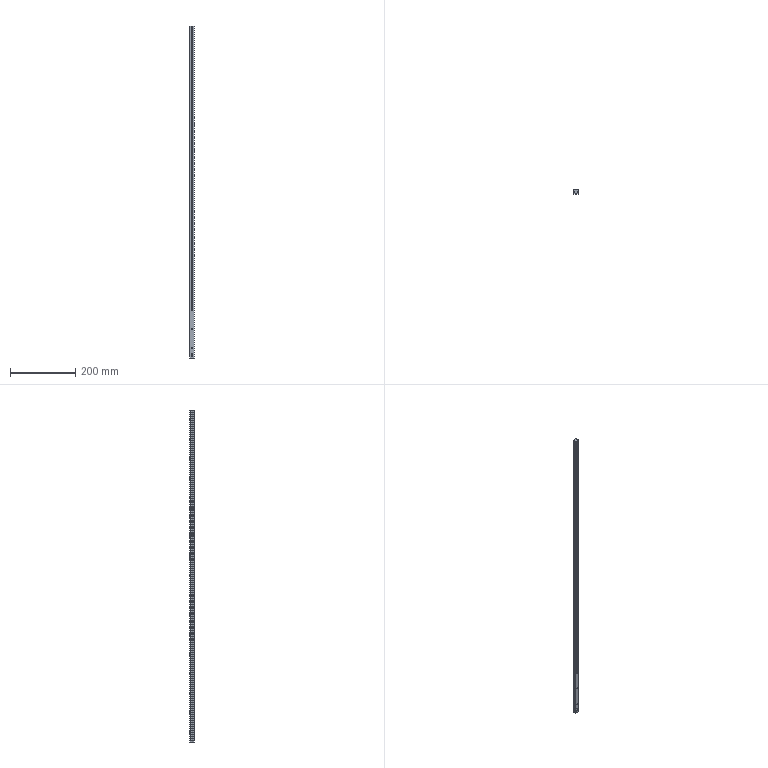Part | SolidWorks | features BaseBody 1, HoleWzd 1, ICE 1, MoveFace 1 | 1 solid | 127 faces | box 15 x 12.5 x 1020 mm | volume 163723 mm3 | cylinder 86 | plane 41 | commonest cylinder face diameters 3.4 x34 6 x34 0.6 x11 3 x5 1 x2